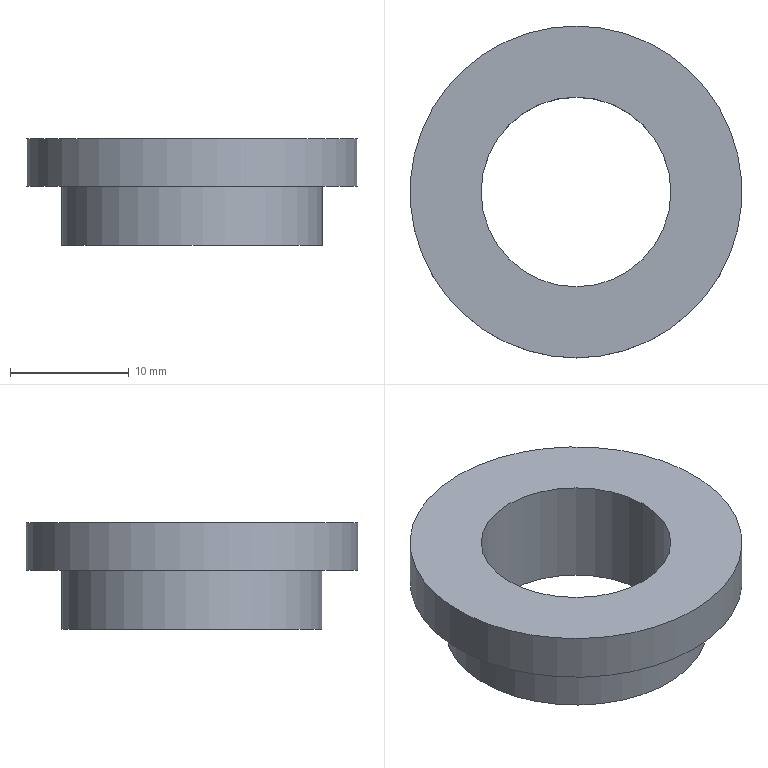Part | STEP file | 1-56.6 | 1 solid | 6 faces | box 28 x 28 x 9 mm | volume 2554 mm3 | plane 3 | cylinder 3 | commonest cylinder face diameters 16 x1 22 x1 28 x1
STEP:
#1=CARTESIAN_POINT('',(0.,0.,0.));
#2=DIRECTION('',(0.,0.,1.));
#3=DIRECTION('',(1.,0.,0.));
#4=AXIS2_PLACEMENT_3D('',#1,#2,#3);
#5=CARTESIAN_POINT('',(0.,11.,-5.));
#6=VERTEX_POINT('',#5);
#7=CARTESIAN_POINT('',(0.,0.,-5.));
#8=DIRECTION('',(0.,0.,1.));
#9=DIRECTION('',(0.,1.,0.));
#10=AXIS2_PLACEMENT_3D('',#7,#8,#9);
#11=CIRCLE('',#10,11.);
#12=CARTESIAN_POINT('',(0.,-2.947,-5.));
#13=DIRECTION('',(0.,0.,1.));
#14=DIRECTION('',(1.,0.,0.));
#15=AXIS2_PLACEMENT_3D('',#12,#13,#14);
#16=PLANE('',#15);
#17=CARTESIAN_POINT('',(0.,2.947));
#18=DIRECTION('',(0.,1.));
#19=AXIS2_PLACEMENT_2D('',#17,#18);
#20=CIRCLE('',#19,11.);
#21=(GEOMETRIC_REPRESENTATION_CONTEXT(2)PARAMETRIC_REPRESENTATION_CONTEXT()REPRESENTATION_CONTEXT('',''));
#22=DEFINITIONAL_REPRESENTATION('',(#20),#21);
#23=PCURVE('',#16,#22);
#24=CARTESIAN_POINT('',(0.,0.,0.));
#25=DIRECTION('',(0.,0.,-1.));
#26=DIRECTION('',(0.,1.,0.));
#27=AXIS2_PLACEMENT_3D('',#24,#25,#26);
#28=CYLINDRICAL_SURFACE('',#27,11.);
#29=CARTESIAN_POINT('',(6.283,5.));
#30=DIRECTION('',(-1.,0.));
#31=VECTOR('',#30,1.);
#32=LINE('',#29,#31);
#33=(GEOMETRIC_REPRESENTATION_CONTEXT(2)PARAMETRIC_REPRESENTATION_CONTEXT()REPRESENTATION_CONTEXT('',''));
#34=DEFINITIONAL_REPRESENTATION('',(#32),#33);
#35=PCURVE('',#28,#34);
#36=SURFACE_CURVE('',#11,(#23,#35),.PCURVE_S1.);
#37=EDGE_CURVE('',#6,#6,#36,.T.);
#38=ORIENTED_EDGE('',*,*,#37,.T.);
#39=EDGE_LOOP('',(#38));
#40=FACE_BOUND('',#39,.F.);
#41=CARTESIAN_POINT('',(0.,8.,-5.));
#42=VERTEX_POINT('',#41);
#43=CARTESIAN_POINT('',(0.,0.,-5.));
#44=DIRECTION('',(0.,0.,-1.));
#45=DIRECTION('',(0.,1.,0.));
#46=AXIS2_PLACEMENT_3D('',#43,#44,#45);
#47=CIRCLE('',#46,8.);
#48=CARTESIAN_POINT('',(0.,10.947));
#49=CARTESIAN_POINT('',(13.856,10.947));
#50=CARTESIAN_POINT('',(6.928,-1.053));
#51=CARTESIAN_POINT('',(0.,-13.053));
#52=CARTESIAN_POINT('',(-6.928,-1.053));
#53=CARTESIAN_POINT('',(-13.856,10.947));
#54=CARTESIAN_POINT('',(0.,10.947));
#55=(BOUNDED_CURVE()B_SPLINE_CURVE(2,(#48,#49,#50,#51,#52,#53,#54),.UNSPECIFIED.,.T.,.F.)B_SPLINE_CURVE_WITH_KNOTS((1,2,2,2,2,1),(-2.094,0.,2.094,4.189,6.283,8.378),.UNSPECIFIED.)CURVE()GEOMETRIC_REPRESENTATION_ITEM()RATIONAL_B_SPLINE_CURVE((1.,0.5,1.,0.5,1.,0.5,1.))REPRESENTATION_ITEM(''));
#56=(GEOMETRIC_REPRESENTATION_CONTEXT(2)PARAMETRIC_REPRESENTATION_CONTEXT()REPRESENTATION_CONTEXT('',''));
#57=DEFINITIONAL_REPRESENTATION('',(#55),#56);
#58=PCURVE('',#16,#57);
#59=CARTESIAN_POINT('',(0.,0.,4.));
#60=DIRECTION('',(0.,0.,-1.));
#61=DIRECTION('',(0.,1.,0.));
#62=AXIS2_PLACEMENT_3D('',#59,#60,#61);
#63=CYLINDRICAL_SURFACE('',#62,8.);
#64=CARTESIAN_POINT('',(0.,9.));
#65=DIRECTION('',(1.,0.));
#66=VECTOR('',#65,1.);
#67=LINE('',#64,#66);
#68=(GEOMETRIC_REPRESENTATION_CONTEXT(2)PARAMETRIC_REPRESENTATION_CONTEXT()REPRESENTATION_CONTEXT('',''));
#69=DEFINITIONAL_REPRESENTATION('',(#67),#68);
#70=PCURVE('',#63,#69);
#71=SURFACE_CURVE('',#47,(#58,#70),.PCURVE_S1.);
#72=EDGE_CURVE('',#42,#42,#71,.T.);
#73=ORIENTED_EDGE('',*,*,#72,.T.);
#74=EDGE_LOOP('',(#73));
#75=FACE_BOUND('',#74,.F.);
#76=ADVANCED_FACE('',(#40,#75),#16,.F.);
#77=CARTESIAN_POINT('',(0.,11.,0.));
#78=VERTEX_POINT('',#77);
#79=CARTESIAN_POINT('',(0.,11.,0.));
#80=DIRECTION('',(0.,0.,-1.));
#81=VECTOR('',#80,1.);
#82=LINE('',#79,#81);
#83=CARTESIAN_POINT('',(6.283,0.));
#84=DIRECTION('',(0.,1.));
#85=VECTOR('',#84,1.);
#86=LINE('',#83,#85);
#87=(GEOMETRIC_REPRESENTATION_CONTEXT(2)PARAMETRIC_REPRESENTATION_CONTEXT()REPRESENTATION_CONTEXT('',''));
#88=DEFINITIONAL_REPRESENTATION('',(#86),#87);
#89=PCURVE('',#28,#88);
#90=CARTESIAN_POINT('',(0.,0.));
#91=DIRECTION('',(0.,1.));
#92=VECTOR('',#91,1.);
#93=LINE('',#90,#92);
#94=(GEOMETRIC_REPRESENTATION_CONTEXT(2)PARAMETRIC_REPRESENTATION_CONTEXT()REPRESENTATION_CONTEXT('',''));
#95=DEFINITIONAL_REPRESENTATION('',(#93),#94);
#96=PCURVE('',#28,#95);
#97=SEAM_CURVE('',#82,(#89,#96),.PCURVE_S1.);
#98=EDGE_CURVE('',#78,#6,#97,.T.);
#99=ORIENTED_EDGE('',*,*,#98,.T.);
#100=ORIENTED_EDGE('',*,*,#37,.T.);
#101=ORIENTED_EDGE('',*,*,#98,.F.);
#102=CARTESIAN_POINT('',(0.,0.,0.));
#103=DIRECTION('',(0.,0.,1.));
#104=DIRECTION('',(0.,1.,0.));
#105=AXIS2_PLACEMENT_3D('',#102,#103,#104);
#106=CIRCLE('',#105,11.);
#107=CARTESIAN_POINT('',(6.283,0.));
#108=DIRECTION('',(-1.,0.));
#109=VECTOR('',#108,1.);
#110=LINE('',#107,#109);
#111=(GEOMETRIC_REPRESENTATION_CONTEXT(2)PARAMETRIC_REPRESENTATION_CONTEXT()REPRESENTATION_CONTEXT('',''));
#112=DEFINITIONAL_REPRESENTATION('',(#110),#111);
#113=PCURVE('',#28,#112);
#114=CARTESIAN_POINT('',(0.,-3.751,0.));
#115=DIRECTION('',(0.,0.,1.));
#116=DIRECTION('',(1.,0.,0.));
#117=AXIS2_PLACEMENT_3D('',#114,#115,#116);
#118=PLANE('',#117);
#119=CARTESIAN_POINT('',(0.,3.751));
#120=DIRECTION('',(0.,1.));
#121=AXIS2_PLACEMENT_2D('',#119,#120);
#122=CIRCLE('',#121,11.);
#123=(GEOMETRIC_REPRESENTATION_CONTEXT(2)PARAMETRIC_REPRESENTATION_CONTEXT()REPRESENTATION_CONTEXT('',''));
#124=DEFINITIONAL_REPRESENTATION('',(#122),#123);
#125=PCURVE('',#118,#124);
#126=SURFACE_CURVE('',#106,(#113,#125),.PCURVE_S1.);
#127=EDGE_CURVE('',#78,#78,#126,.T.);
#128=ORIENTED_EDGE('',*,*,#127,.F.);
#129=EDGE_LOOP('',(#99,#100,#101,#128));
#130=FACE_BOUND('',#129,.T.);
#131=ADVANCED_FACE('',(#130),#28,.T.);
#132=ORIENTED_EDGE('',*,*,#72,.F.);
#133=CARTESIAN_POINT('',(0.,8.,4.));
#134=VERTEX_POINT('',#133);
#135=CARTESIAN_POINT('',(0.,8.,-5.));
#136=DIRECTION('',(0.,0.,1.));
#137=VECTOR('',#136,1.);
#138=LINE('',#135,#137);
#139=CARTESIAN_POINT('',(0.,9.));
#140=DIRECTION('',(0.,-1.));
#141=VECTOR('',#140,1.);
#142=LINE('',#139,#141);
#143=(GEOMETRIC_REPRESENTATION_CONTEXT(2)PARAMETRIC_REPRESENTATION_CONTEXT()REPRESENTATION_CONTEXT('',''));
#144=DEFINITIONAL_REPRESENTATION('',(#142),#143);
#145=PCURVE('',#63,#144);
#146=CARTESIAN_POINT('',(6.283,9.));
#147=DIRECTION('',(0.,-1.));
#148=VECTOR('',#147,1.);
#149=LINE('',#146,#148);
#150=(GEOMETRIC_REPRESENTATION_CONTEXT(2)PARAMETRIC_REPRESENTATION_CONTEXT()REPRESENTATION_CONTEXT('',''));
#151=DEFINITIONAL_REPRESENTATION('',(#149),#150);
#152=PCURVE('',#63,#151);
#153=SEAM_CURVE('',#138,(#145,#152),.PCURVE_S1.);
#154=EDGE_CURVE('',#42,#134,#153,.T.);
#155=ORIENTED_EDGE('',*,*,#154,.T.);
#156=CARTESIAN_POINT('',(0.,0.,4.));
#157=DIRECTION('',(0.,0.,-1.));
#158=DIRECTION('',(0.,1.,0.));
#159=AXIS2_PLACEMENT_3D('',#156,#157,#158);
#160=CIRCLE('',#159,8.);
#161=CARTESIAN_POINT('',(0.,0.));
#162=DIRECTION('',(1.,0.));
#163=VECTOR('',#162,1.);
#164=LINE('',#161,#163);
#165=(GEOMETRIC_REPRESENTATION_CONTEXT(2)PARAMETRIC_REPRESENTATION_CONTEXT()REPRESENTATION_CONTEXT('',''));
#166=DEFINITIONAL_REPRESENTATION('',(#164),#165);
#167=PCURVE('',#63,#166);
#168=CARTESIAN_POINT('',(0.,-3.751,4.));
#169=DIRECTION('',(0.,0.,1.));
#170=DIRECTION('',(1.,0.,0.));
#171=AXIS2_PLACEMENT_3D('',#168,#169,#170);
#172=PLANE('',#171);
#173=CARTESIAN_POINT('',(0.,11.751));
#174=CARTESIAN_POINT('',(13.856,11.751));
#175=CARTESIAN_POINT('',(6.928,-0.2487));
#176=CARTESIAN_POINT('',(0.,-12.249));
#177=CARTESIAN_POINT('',(-6.928,-0.2487));
#178=CARTESIAN_POINT('',(-13.856,11.751));
#179=CARTESIAN_POINT('',(0.,11.751));
#180=(BOUNDED_CURVE()B_SPLINE_CURVE(2,(#173,#174,#175,#176,#177,#178,#179),.UNSPECIFIED.,.T.,.F.)B_SPLINE_CURVE_WITH_KNOTS((1,2,2,2,2,1),(-2.094,0.,2.094,4.189,6.283,8.378),.UNSPECIFIED.)CURVE()GEOMETRIC_REPRESENTATION_ITEM()RATIONAL_B_SPLINE_CURVE((1.,0.5,1.,0.5,1.,0.5,1.))REPRESENTATION_ITEM(''));
#181=(GEOMETRIC_REPRESENTATION_CONTEXT(2)PARAMETRIC_REPRESENTATION_CONTEXT()REPRESENTATION_CONTEXT('',''));
#182=DEFINITIONAL_REPRESENTATION('',(#180),#181);
#183=PCURVE('',#172,#182);
#184=SURFACE_CURVE('',#160,(#167,#183),.PCURVE_S1.);
#185=EDGE_CURVE('',#134,#134,#184,.T.);
#186=ORIENTED_EDGE('',*,*,#185,.T.);
#187=ORIENTED_EDGE('',*,*,#154,.F.);
#188=EDGE_LOOP('',(#132,#155,#186,#187));
#189=FACE_BOUND('',#188,.F.);
#190=ADVANCED_FACE('',(#189),#63,.F.);
#191=CARTESIAN_POINT('',(0.,14.,0.));
#192=VERTEX_POINT('',#191);
#193=CARTESIAN_POINT('',(0.,0.,0.));
#194=DIRECTION('',(0.,0.,1.));
#195=DIRECTION('',(0.,1.,0.));
#196=AXIS2_PLACEMENT_3D('',#193,#194,#195);
#197=CIRCLE('',#196,14.);
#198=CARTESIAN_POINT('',(0.,3.751));
#199=DIRECTION('',(0.,1.));
#200=AXIS2_PLACEMENT_2D('',#198,#199);
#201=CIRCLE('',#200,14.);
#202=(GEOMETRIC_REPRESENTATION_CONTEXT(2)PARAMETRIC_REPRESENTATION_CONTEXT()REPRESENTATION_CONTEXT('',''));
#203=DEFINITIONAL_REPRESENTATION('',(#201),#202);
#204=PCURVE('',#118,#203);
#205=CARTESIAN_POINT('',(0.,0.,0.));
#206=DIRECTION('',(0.,0.,1.));
#207=DIRECTION('',(0.,1.,0.));
#208=AXIS2_PLACEMENT_3D('',#205,#206,#207);
#209=CYLINDRICAL_SURFACE('',#208,14.);
#210=CARTESIAN_POINT('',(0.,0.));
#211=DIRECTION('',(1.,0.));
#212=VECTOR('',#211,1.);
#213=LINE('',#210,#212);
#214=(GEOMETRIC_REPRESENTATION_CONTEXT(2)PARAMETRIC_REPRESENTATION_CONTEXT()REPRESENTATION_CONTEXT('',''));
#215=DEFINITIONAL_REPRESENTATION('',(#213),#214);
#216=PCURVE('',#209,#215);
#217=SURFACE_CURVE('',#197,(#204,#216),.PCURVE_S1.);
#218=EDGE_CURVE('',#192,#192,#217,.T.);
#219=ORIENTED_EDGE('',*,*,#218,.T.);
#220=EDGE_LOOP('',(#219));
#221=FACE_BOUND('',#220,.F.);
#222=ORIENTED_EDGE('',*,*,#127,.F.);
#223=EDGE_LOOP('',(#222));
#224=FACE_BOUND('',#223,.F.);
#225=ADVANCED_FACE('',(#221,#224),#118,.F.);
#226=ORIENTED_EDGE('',*,*,#218,.T.);
#227=CARTESIAN_POINT('',(0.,14.,4.));
#228=VERTEX_POINT('',#227);
#229=CARTESIAN_POINT('',(0.,14.,0.));
#230=DIRECTION('',(0.,0.,1.));
#231=VECTOR('',#230,1.);
#232=LINE('',#229,#231);
#233=CARTESIAN_POINT('',(6.283,0.));
#234=DIRECTION('',(0.,1.));
#235=VECTOR('',#234,1.);
#236=LINE('',#233,#235);
#237=(GEOMETRIC_REPRESENTATION_CONTEXT(2)PARAMETRIC_REPRESENTATION_CONTEXT()REPRESENTATION_CONTEXT('',''));
#238=DEFINITIONAL_REPRESENTATION('',(#236),#237);
#239=PCURVE('',#209,#238);
#240=CARTESIAN_POINT('',(0.,0.));
#241=DIRECTION('',(0.,1.));
#242=VECTOR('',#241,1.);
#243=LINE('',#240,#242);
#244=(GEOMETRIC_REPRESENTATION_CONTEXT(2)PARAMETRIC_REPRESENTATION_CONTEXT()REPRESENTATION_CONTEXT('',''));
#245=DEFINITIONAL_REPRESENTATION('',(#243),#244);
#246=PCURVE('',#209,#245);
#247=SEAM_CURVE('',#232,(#239,#246),.PCURVE_S1.);
#248=EDGE_CURVE('',#192,#228,#247,.T.);
#249=ORIENTED_EDGE('',*,*,#248,.T.);
#250=CARTESIAN_POINT('',(0.,0.,4.));
#251=DIRECTION('',(0.,0.,1.));
#252=DIRECTION('',(0.,1.,0.));
#253=AXIS2_PLACEMENT_3D('',#250,#251,#252);
#254=CIRCLE('',#253,14.);
#255=CARTESIAN_POINT('',(0.,4.));
#256=DIRECTION('',(1.,0.));
#257=VECTOR('',#256,1.);
#258=LINE('',#255,#257);
#259=(GEOMETRIC_REPRESENTATION_CONTEXT(2)PARAMETRIC_REPRESENTATION_CONTEXT()REPRESENTATION_CONTEXT('',''));
#260=DEFINITIONAL_REPRESENTATION('',(#258),#259);
#261=PCURVE('',#209,#260);
#262=CARTESIAN_POINT('',(0.,3.751));
#263=DIRECTION('',(0.,1.));
#264=AXIS2_PLACEMENT_2D('',#262,#263);
#265=CIRCLE('',#264,14.);
#266=(GEOMETRIC_REPRESENTATION_CONTEXT(2)PARAMETRIC_REPRESENTATION_CONTEXT()REPRESENTATION_CONTEXT('',''));
#267=DEFINITIONAL_REPRESENTATION('',(#265),#266);
#268=PCURVE('',#172,#267);
#269=SURFACE_CURVE('',#254,(#261,#268),.PCURVE_S1.);
#270=EDGE_CURVE('',#228,#228,#269,.T.);
#271=ORIENTED_EDGE('',*,*,#270,.F.);
#272=ORIENTED_EDGE('',*,*,#248,.F.);
#273=EDGE_LOOP('',(#226,#249,#271,#272));
#274=FACE_BOUND('',#273,.T.);
#275=ADVANCED_FACE('',(#274),#209,.T.);
#276=ORIENTED_EDGE('',*,*,#270,.T.);
#277=EDGE_LOOP('',(#276));
#278=FACE_BOUND('',#277,.T.);
#279=ORIENTED_EDGE('',*,*,#185,.T.);
#280=EDGE_LOOP('',(#279));
#281=FACE_BOUND('',#280,.T.);
#282=ADVANCED_FACE('',(#278,#281),#172,.T.);
#283=CLOSED_SHELL('',(#76,#131,#190,#225,#275,#282));
#284=MANIFOLD_SOLID_BREP('',#283);
#285=(LENGTH_UNIT()NAMED_UNIT(*)SI_UNIT(.MILLI.,.METRE.));
#286=UNCERTAINTY_MEASURE_WITH_UNIT(LENGTH_MEASURE(0.0000001),#285,'','');
#287=(NAMED_UNIT(*)PLANE_ANGLE_UNIT()SI_UNIT($,.RADIAN.));
#288=(NAMED_UNIT(*)SI_UNIT($,.STERADIAN.)SOLID_ANGLE_UNIT());
#289=(GEOMETRIC_REPRESENTATION_CONTEXT(3)GLOBAL_UNCERTAINTY_ASSIGNED_CONTEXT((#286))GLOBAL_UNIT_ASSIGNED_CONTEXT((#285,#287,#288))REPRESENTATION_CONTEXT('',''));
#290=ADVANCED_BREP_SHAPE_REPRESENTATION('',(#4,#284),#289);